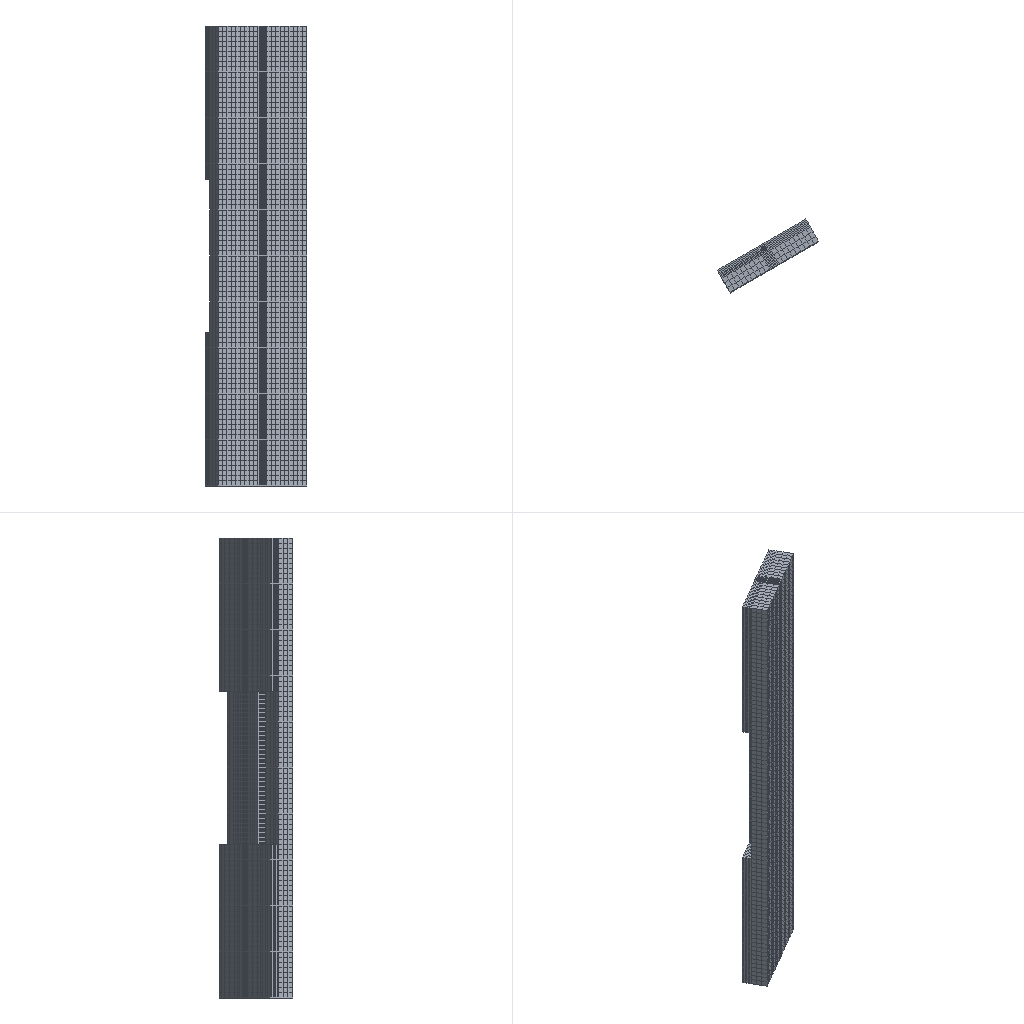Simulation study | abaqus
Set-up summary:
category,name,step,type,value,unit,region
solver,abaqus
solver,version,,,Abaqus/Standard 2020
units,not stated in the deck,,not stated
analysis,deck,,transient,transient
load_step,Gravity,Gravity,transient
load_step,requested,,,1
mesh,nodes,,,35489
mesh,elements,,,27780
element_type,C3D8,,solid,27780
load,load commands in deck,,count,3
bc,support commands in deck,,count,13
material,MAT-HUACHUANG,,in results
material,MAT-PIPE,,in results
material,MATE-HUATI,,in results
check,setup vs results,,match,"per instance, exact: element labels, types and connectivity; labels of the nodes the elements use; coordinates of those nodes at SINGLE_PRECISION in 3 of 3 instance(s)"
Abaqus input file, long lists of numbers shortened:
*Heading
** Job name: Job-1 Model name: Model-1
** Generated by: Abaqus/CAE 2020
*Preprint, echo=NO, model=NO, history=NO, contact=NO
**
** PARTS
**
*Part, name=huachuang
*End Part
**
*Part, name=huati
*End Part
**
*Part, name=pipe
*End Part
**
**
** ASSEMBLY
**
*Assembly, name=Assembly
**
*Instance, name=huachuang-1, part=huachuang
          0.,           0.,           0.
          0.,           0.,           0.,           0.,           0., 1., 30.
*Node
      1,           7.,   8.2,         120.
      2,           7.,   8.2,         180.
** (21823 more lines like these left out)
*Element, type=C3D8
  1,   246,  2747, 12140,  2715,     1,    95,  2251,   168
  2,  2747,  2748, 12141, 12140,    95,    96,  2252,  2251
** (17698 more lines like these left out)
*Nset, nset=_PickedSet97, internal, generate
     1,  21825,      1
*Elset, elset=_PickedSet97, internal, generate
     1,  17700,      1
*Elset, elset=_Surf-huachuang_S2, internal
  8191,  8192,  8193,  8194,  8195,  8196,  8197,  8198,  8199,  8200,  8201,  8202,  8203,  8204,  8205,  8206
  8207,  8208,  8209,  8210,  8211,  8212,  8213,  8214,  8215,  8216,  8217,  8218,  8219,  8220,  8221,  8222
** (21 more lines like these left out)
*Elset, elset=_Surf-huachuang_S5, internal
 3961, 3962, 3963, 3964, 3965, 3966, 3967, 3968, 3969, 3970, 3971, 3972, 3973, 3974, 3975, 3976
 3977, 3978, 3979, 3980, 3981, 3982, 3983, 3984, 3985, 3986, 3987, 3988, 3989, 3990, 4231, 4232
** (4 more lines like these left out)
*Surface, type=ELEMENT, name=Surf-huachuang
_Surf-huachuang_S2, S2
_Surf-huachuang_S5, S5
** Section: Section-huachuang
*Solid Section, elset=_PickedSet97, material=Mat-huachuang
,
*End Instance
**
*Instance, name=pipe-1, part=pipe
0.2301, 9.601,           0.
0.2301, 9.601,           0., 0.2301, 9.601, 1., 30.
*Node
      1,  0.5911,           0.,           0.
      2,  0.5911,           0.,         180.
** (2438 more lines like these left out)
*Element, type=C3D8
  1,    8,  203,  789,  267,    1,   19,  553,  144
  2,  203,  202,  790,  789,   19,   20,  554,  553
** (1198 more lines like these left out)
*Nset, nset=Set-pipe, generate
    1,  2440,     1
*Elset, elset=Set-pipe, generate
    1,  1200,     1
** Section: Section-pipe
*Solid Section, elset=Set-pipe, material=Mat-pipe
,
*End Instance
**
*Instance, name=huati-1, part=huati
          0.,           0.,           0.
          0.,           0.,           0.,           0.,           0., 1., 30.
*Node
      1,           7.,          10.,         120.
      2,           7.,   8.2,         120.
** (11222 more lines like these left out)
*Element, type=C3D8
  1, 1393, 1394, 6416, 6387,   66,   67, 1268, 1267
  2, 1394, 1395, 6415, 6416,   67,   68, 1269, 1268
** (8878 more lines like these left out)
*Nset, nset=Set-23, generate
     1,  11224,      1
*Elset, elset=Set-23, generate
    1,  8880,     1
** Section: Section-huati
*Solid Section, elset=Set-23, material=Mate-huati
,
*End Instance
**
*Nset, nset=Set-9, instance=pipe-1, generate
    1,  2440,     1
*Elset, elset=Set-9, instance=pipe-1, generate
    1,  1200,     1
*Nset, nset=Set-Huati, instance=huati-1, generate
     1,  11224,      1
*Elset, elset=Set-Huati, instance=huati-1, generate
    1,  8880,     1
*Nset, nset=Set-Huati-Side, instance=huati-1
    1,    2,    3,    4,    5,    6,    7,    8,    9,   10,   11,   12,   13,   14,   15,   16
   17,   18,   19,   20,   21,   22,   23,   24,   25,   26,   27,   28,   29,   30,   31,   32
** (21 more lines like these left out)
*Elset, elset=Set-Huati-Side, instance=huati-1
   30,   31,   32,  120,  150,  151,  181,  182,  183,  271,  272,  273,  274,  275,  276,  451
  452,  453,  454,  571,  572,  573,  661,  662,  663,  664,  781,  782,  783,  784,  785,  786
** (17 more lines like these left out)
*Nset, nset=Set-cemian, instance=huachuang-1
     2,     3,     5,     6,    10,    11,    13,    14,    22,    23,    25,    28,    29,    30,    31,    32
    34,    35,    38,    39,    42,    44,    46,    47,    48,    49,    50,    55,    58,    59,    62,    64
** (36 more lines like these left out)
*Nset, nset=Set-cemian, instance=pipe-1
   1,   2,   3,   4,   5,   6,   7,   8,   9,  10,  11,  12,  13,  14,  15,  16
  17,  18,  78,  79,  80,  81, 141, 142, 143, 144, 204, 205, 206, 207, 267, 268
** (3 more lines like these left out)
*Elset, elset=Set-cemian, instance=huachuang-1
    30,    60,    90,   120,   150,   180,   210,   240,   270,   300,   330,   360,   390,   420,   450,   480
   510,   540,   570,   600,   630,   660,   690,   720,   750,   780,   810,   840,   870,   900,   930,   960
** (30 more lines like these left out)
*Elset, elset=Set-cemian, instance=pipe-1
    1,   60,   61,  120,  121,  180,  181,  240,  241,  300,  301,  360,  361,  420,  421,  480
  481,  540,  541,  600,  601,  660,  661,  720,  721,  780,  781,  840,  841,  900,  901,  960
** (1 more lines like these left out)
*Nset, nset=Set-dimian, instance=huachuang-1
    17,    18,    19,    20,    29,    30,    31,    32,    47,    50,    51,    54,    59,    60,    61,    62
    87,    88,    91,    92,   465,   466,   467,   468,   469,   470,   471,   472,   473,   474,   475,   476
** (152 more lines like these left out)
*Elset, elset=Set-dimian, instance=huachuang-1
  2161,  2162,  2163,  2164,  2165,  2166,  2167,  2168,  2169,  2170,  2171,  2172,  2173,  2174,  2175,  2176
  2177,  2178,  2179,  2180,  2181,  2182,  2183,  2184,  2185,  2186,  2187,  2188,  2189,  2190,  2191,  2192
** (145 more lines like these left out)
*Nset, nset=Set-load, instance=huati-1
   11,   12,   15,   16,   35,   36,  358,  359,  360,  361,  362,  363,  364,  365,  366,  367
  368,  369,  370,  371,  372,  373,  374,  375,  376,  377,  378,  379,  380,  381,  382,  383
** (29 more lines like these left out)
*Elset, elset=Set-load, instance=huati-1
  961,  962,  963,  964,  965,  966,  967,  968,  969,  970,  971,  972,  973,  974,  975,  976
  977,  978,  979,  980,  981,  982,  983,  984,  985,  986,  987,  988,  989,  990,  991,  992
** (25 more lines like these left out)
*Nset, nset=Set-qianmian, instance=huachuang-1
     3,     4,     6,     7,    11,    12,    14,    15,    18,    19,    30,    32,    35,    36,    69,    70
    71,    72,    73,    74,    75,    76,    82,    83,    87,    88,    89,    90,    91,    92,    93,    94
** (92 more lines like these left out)
*Elset, elset=Set-qianmian, instance=huachuang-1
   241,   242,   243,   244,   245,   246,   247,   248,   249,   250,   251,   252,   253,   254,   255,   256
   257,   258,   259,   260,   261,   262,   263,   264,   265,   266,   267,   268,   269,   270,   511,   512
** (79 more lines like these left out)
*Nset, nset=huachuang, instance=huachuang-1, generate
     1,  21825,      1
*Elset, elset=huachuang, instance=huachuang-1, generate
     1,  17700,      1
*Nset, nset=model-all, instance=huachuang-1, generate
     1,  21825,      1
*Nset, nset=model-all, instance=pipe-1, generate
    1,  2440,     1
*Nset, nset=model-all, instance=huati-1, generate
     1,  11224,      1
*Elset, elset=model-all, instance=huachuang-1, generate
     1,  17700,      1
*Elset, elset=model-all, instance=pipe-1, generate
    1,  1200,     1
*Elset, elset=model-all, instance=huati-1, generate
    1,  8880,     1
*Elset, elset=_Huachuang-mid-top_S2, internal, instance=huachuang-1
  1621,  1622,  1623,  1624,  1625,  1626,  1627,  1628,  1629,  1630,  1631,  1632,  1633,  1634,  1635,  1636
  1637,  1638,  1639,  1640,  1641,  1642,  1643,  1644,  1645,  1646,  1647,  1648,  1649,  1650,  1651,  1652
** (23 more lines like these left out)
*Elset, elset=_Huachuang-mid-top_S6, internal, instance=huachuang-1, generate
 13171,  13978,      3
*Elset, elset=_Huachuang-mid-top_S1, internal, instance=huachuang-1, generate
 7261,  7380,     1
*Surface, type=ELEMENT, name=Huachuang-mid-top
_Huachuang-mid-top_S2, S2
_Huachuang-mid-top_S6, S6
_Huachuang-mid-top_S1, S1
*Elset, elset=_Huati-bottom_S2, internal, instance=huati-1
  961,  962,  963,  964,  965,  966,  967,  968,  969,  970,  971,  972,  973,  974,  975,  976
  977,  978,  979,  980,  981,  982,  983,  984,  985,  986,  987,  988,  989,  990,  991,  992
** (43 more lines like these left out)
*Elset, elset=_Huati-bottom_S3, internal, instance=huati-1
 5101, 5102, 5103, 5104, 5105, 5106, 5107, 5108, 5109, 5110, 5111, 5112, 5113, 5114, 5115, 5116
 5117, 5118, 5119, 5120, 5121, 5122, 5123, 5124, 5125, 5126, 5127, 5128, 5129, 5130, 5131, 5132
** (10 more lines like these left out)
*Elset, elset=_Huati-bottom_S4, internal, instance=huati-1
 4801, 4802, 4803, 4804, 4805, 4806, 4807, 4808, 4809, 4810, 4811, 4812, 4813, 4814, 4815, 4816
 4817, 4818, 4819, 4820, 4821, 4822, 4823, 4824, 4825, 4826, 4827, 4828, 4829, 4830, 4831, 4832
** (10 more lines like these left out)
*Surface, type=ELEMENT, name=Huati-bottom
_Huati-bottom_S2, S2
_Huati-bottom_S3, S3
_Huati-bottom_S4, S4
*Elset, elset=_Surf-13_S2, internal, instance=pipe-1, generate
 301,  900,    1
*Surface, type=ELEMENT, name=Surf-13
_Surf-13_S2, S2
*Elset, elset=_Surf-LOAD_S3, internal, instance=huati-1
  961,  962,  963,  964,  965,  966,  967,  968,  969,  970,  971,  972,  973,  974,  975,  976
  977,  978,  979,  980,  981,  982,  983,  984,  985,  986,  987,  988,  989,  990,  991,  992
** (25 more lines like these left out)
*Surface, type=ELEMENT, name=Surf-LOAD
_Surf-LOAD_S3, S3
*Elset, elset=_Surf-huachuang_S4, internal, instance=huachuang-1
  9392,  9394,  9396,  9398,  9400,  9402,  9404,  9406,  9408,  9410,  9412,  9414,  9416,  9418,  9420,  9422
  9424,  9426,  9428,  9430,  9432,  9434,  9436,  9438,  9440,  9442,  9444,  9446,  9448,  9450, 10562, 10564
** (18 more lines like these left out)
*Elset, elset=_Surf-huachuang_S3, internal, instance=huachuang-1
  9331,  9332,  9333,  9334,  9335,  9336,  9337,  9338,  9339,  9340,  9341,  9342,  9343,  9344,  9345,  9361
  9362,  9363,  9364,  9365,  9366,  9367,  9368,  9369,  9370,  9371,  9372,  9373,  9374,  9375,  9481,  9482
** (16 more lines like these left out)
*Elset, elset=_Surf-huachuang_S2, internal, instance=huachuang-1
  2431,  2432,  2433,  2434,  2435,  2436,  2437,  2438,  2439,  2440,  2441,  2442,  2443,  2444,  2445,  2446
  2447,  2448,  2449,  2450,  2451,  2452,  2453,  2454,  2455,  2456,  2457,  2458,  2459,  2460,  2461,  2462
** (35 more lines like these left out)
*Elset, elset=_Surf-huachuang_S6, internal, instance=huachuang-1, generate
 12931,  13019,      2
*Surface, type=ELEMENT, name=Surf-huachuang
_Surf-huachuang_S4, S4
_Surf-huachuang_S3, S3
_Surf-huachuang_S2, S2
_Surf-huachuang_S6, S6
*Elset, elset=_Surf-huati_S3, internal, instance=huati-1
  451,  452,  455,  456,  459,  460,  463,  464,  467,  468,  471,  472,  475,  476,  479,  480
  483,  484,  487,  488,  491,  492,  495,  496,  499,  500,  503,  504,  507,  508,  511,  512
** (42 more lines like these left out)
*Elset, elset=_Surf-huati_S4, internal, instance=huati-1
  272,  274,  276,  278,  280,  282,  284,  286,  288,  290,  292,  294,  296,  298,  300,  302
  304,  306,  308,  310,  312,  314,  316,  318,  320,  322,  324,  326,  328,  330,  332,  334
** (30 more lines like these left out)
*Surface, type=ELEMENT, name=Surf-huati
_Surf-huati_S3, S3
_Surf-huati_S4, S4
*Elset, elset=_Surf-pipe_S1, internal, instance=pipe-1, generate
    1,  1200,     1
*Surface, type=ELEMENT, name=Surf-pipe
_Surf-pipe_S1, S1
*Elset, elset=_huachuang-left-side_S3, internal, instance=huachuang-1
  5341,  5342,  5343,  5386,  5387,  5388,  5641,  5656,  5671,  5731,  5761,  5762,  9301,  9316,  9451, 10471
 10486, 10501, 10741, 14821, 14822, 15121, 15122, 15151, 15152, 16891, 16892, 16893, 16981, 16982, 16983, 17071
** (2 more lines like these left out)
*Elset, elset=_huachuang-left-side_S4, internal, instance=huachuang-1
  5595,  5610,  5625,  5640,  8220,  8250,  8280,  8310,  8340,  8370,  8400,  8430,  8460,  8490,  8520,  8550
  8580,  8610,  8640,  8670,  8700,  8730,  8760,  8790,  8820,  8850,  8880,  8910,  8940,  8970,  9000,  9030
** (2 more lines like these left out)
*Elset, elset=_huachuang-left-side_S2, internal, instance=huachuang-1
  9481,  9482,  9483,  9484,  9485,  9486,  9571,  9572,  9573, 10771, 10772, 10773, 10774, 10775, 10776, 10861
 10862, 10863, 15181, 15182, 15183, 15184, 15185, 15186
*Elset, elset=_huachuang-left-side_S6, internal, instance=huachuang-1
    1,   31,   61,   91,  121,  151,  181,  211,  241,  271,  301,  331,  361,  391,  421,  451
  481,  511,  541,  571,  601,  631,  661,  691,  721,  751,  781, 4531, 4561, 4591, 4621, 4651
** (2 more lines like these left out)
*Surface, type=ELEMENT, name=huachuang-left-side
_huachuang-left-side_S3, S3
_huachuang-left-side_S4, S4
_huachuang-left-side_S2, S2
_huachuang-left-side_S6, S6
*Elset, elset=_huachuang-right-side_S3, internal, instance=huachuang-1
  2431,  2432,  2433,  2476,  2477,  2478,  2776,  2791,  2806,  6721,  6722,  6751,  6752, 12211, 12226, 12391
 12721, 12722, 13021, 13022, 13051, 13052
*Elset, elset=_huachuang-right-side_S4, internal, instance=huachuang-1
  2685,  2700,  2715,  2730,  6645,  6660,  6675,  6690,  6705,  6720,  6900,  6915,  6930,  7410,  7440,  7470
  7500,  7530,  7560,  7590,  7620,  7650,  7680,  7710,  7740,  7770,  7800,  7830,  7860,  7890,  7920,  7950
** (3 more lines like these left out)
*Elset, elset=_huachuang-right-side_S2, internal, instance=huachuang-1
  2821,  2822,  2851,  6931,  6946,  6947, 12421, 12422, 12423, 12424, 12425, 12426, 12511, 12512, 12513, 13081
 13082, 13083, 13084, 13085, 13086
*Elset, elset=_huachuang-right-side_S6, internal, instance=huachuang-1
   811,   841,   871,   901,   931,   961,   991,  1021,  1051,  1081,  1111,  1141,  1171,  1201,  1231,  1261
  1291,  1321,  1351,  1381,  1411,  1441,  1471,  1501,  1531,  1561,  1591, 13981, 14011, 14041, 14071, 14101
** (2 more lines like these left out)
*Surface, type=ELEMENT, name=huachuang-right-side
_huachuang-right-side_S3, S3
_huachuang-right-side_S4, S4
_huachuang-right-side_S2, S2
_huachuang-right-side_S6, S6
*Elset, elset=_huati-left-side_S4, internal, instance=huati-1
   30, 1020, 1080, 1140, 1200, 1260, 1320, 1380, 1440, 1500, 1560, 1620, 1680, 1740, 1800, 1860
 1920, 1980, 2040, 2100, 2160, 2220, 2280, 2340, 2400, 3960, 3990, 5130, 5160, 5490, 5520, 5550
** (2 more lines like these left out)
*Elset, elset=_huati-left-side_S3, internal, instance=huati-1
   31,   32, 3991, 4411, 4412, 4413, 4981, 4982, 5041, 5042, 5551, 8221, 8251, 8611, 8612, 8613
*Elset, elset=_huati-left-side_S2, internal, instance=huati-1
  181,  182,  183,  271,  272,  273,  274,  275,  276,  451,  452,  453,  454, 4501, 4502, 4503
 4504, 4621, 4622, 4623, 4624, 4625, 4626, 8701, 8702, 8703, 8704, 8705, 8706
*Elset, elset=_huati-left-side_S6, internal, instance=huati-1
 2401, 2461, 2521, 2581, 2641, 2701, 2761, 2821, 2881, 2941, 3001, 3061, 3121, 3181, 3241, 3301
 3361, 3421, 3481, 3541, 3601, 3661, 3721, 3781, 6841, 6901, 6961, 7021, 7081, 7141, 7201, 7261
** (1 more lines like these left out)
*Surface, type=ELEMENT, name=huati-left-side
_huati-left-side_S4, S4
_huati-left-side_S3, S3
_huati-left-side_S2, S2
_huati-left-side_S6, S6
*Elset, elset=_huati-right-side_S4, internal, instance=huati-1
  120,  150, 2460, 2520, 2580, 2640, 2700, 2760, 2820, 2880, 2940, 3000, 3060, 3120, 3180, 3240
 3300, 3360, 3420, 3480, 3540, 3600, 3660, 3720, 3780, 3840, 3870, 4890, 4920, 4950, 4980, 6900
** (2 more lines like these left out)
*Elset, elset=_huati-right-side_S6, internal, instance=huati-1
  961, 1021, 1081, 1141, 1201, 1261, 1321, 1381, 1441, 1501, 1561, 1621, 1681, 1741, 1801, 1861
 1921, 1981, 2041, 2101, 2161, 2221, 2281, 2341, 5761, 5821, 5881, 5941, 6001, 6061, 6121, 6181
** (1 more lines like these left out)
*Elset, elset=_huati-right-side_S3, internal, instance=huati-1
  151,  571,  572,  573, 3871, 3872, 4801, 4831, 7981, 7982, 8041, 8042
*Elset, elset=_huati-right-side_S2, internal, instance=huati-1
  661,  662,  663,  664,  781,  782,  783,  784,  785,  786, 4021, 4022, 4023, 4111, 4112, 4113
 4114, 4115, 4116, 4291, 4292, 4293, 4294, 5161, 5162, 5163, 5164, 5165, 5166, 5341, 5342, 5343
** (1 more lines like these left out)
*Surface, type=ELEMENT, name=huati-right-side
_huati-right-side_S4, S4
_huati-right-side_S6, S6
_huati-right-side_S2, S2
_huati-right-side_S3, S3
*Elset, elset=_pipe-inner_S2, internal, instance=pipe-1, generate
    1,  1200,     1
*Surface, type=ELEMENT, name=pipe-inner
_pipe-inner_S2, S2
*End Assembly
*Amplitude, name=Amp-1
             0.,              0.,              1.,              1.
**
** MATERIALS
**
*Material, name=Mat-huachuang
*Density
1800.,
*Elastic
 3.2e+06, 0.28
*Mohr Coulomb
20., 0.1
*Mohr Coulomb Hardening
 2e+07,0.
*Material, name=Mat-pipe
*Density
7900.,
*Elastic
 2.1e+11, 0.3
*Expansion
 1.25e-05,
*Plastic
 4.60095e+08,          0.
 4.67441e+08,    8.87e-06
 4.74118e+08,    1.63e-05
 4.80796e+08,    2.73e-05
 4.87474e+08,    4.35e-05
 4.94152e+08,    6.72e-05
 5.00829e+08, 0.0001015
 5.07507e+08, 0.000151
 5.14185e+08,   0.0002218
 5.20862e+08, 0.0003226
  5.2754e+08, 0.000465
 5.34218e+08, 0.0006646
 5.40896e+08, 0.0009423
 5.47573e+08,  0.001325
 5.54251e+08,   0.001846
 5.60929e+08,  0.002547
 5.67607e+08,  0.003475
 5.74284e+08,  0.004684
 5.80962e+08,  0.006226
  5.8764e+08,  0.008154
 5.94317e+08,   0.01051
 6.00995e+08,   0.01331
 6.07673e+08,   0.01658
 6.14351e+08,   0.02031
 6.21028e+08,   0.02448
 6.27706e+08,   0.02906
 6.34384e+08,   0.03401
 6.41061e+08,   0.03929
 6.47739e+08,   0.04486
 6.54417e+08,   0.05071
 6.61095e+08,   0.05683
 6.67772e+08,   0.06302
*Material, name=Mate-huati
*Density
1800.,
*Elastic
 3.115e+06, 0.3
*Mohr Coulomb
20., 0.1
*Mohr Coulomb Hardening
 2e+07,0.
**
** INTERACTION PROPERTIES
**
*Surface Interaction, name=IntProp-1
1.,
*Friction, slip tolerance=0.005
 0.3,
*Surface Behavior, pressure-overclosure=HARD
**
** BOUNDARY CONDITIONS
**
** Name: huachuang-cemian Type: Displacement/rotation angle
*Boundary
Set-cemian, 1, 1
Set-cemian, 3, 3
** Name: huachuang-dimian Type: Displacement/rotation angle
*Boundary
Set-dimian, 1, 1
Set-dimian, 2, 2
Set-dimian, 3, 3
** Name: huachuang-qianmian Type: Displacement/rotation angle
*Boundary
Set-qianmian, 1, 1
** Name: huati-beimian Type: Displacement/rotation angle
*Boundary
Set-load, 1, 1
**
** PREDEFINED FIELDS
**
** Name: Predefined Field-1   Type: Temperature
*Initial Conditions, type=TEMPERATURE
Set-9, 0.
**
** INTERACTIONS
**
** Interaction: Huachuang-Huati
*Contact Pair, interaction=IntProp-1, type=SURFACE TO SURFACE
Huati-bottom, Huachuang-mid-top
** Interaction: huachuang-huati-left-side
*Contact Pair, interaction=IntProp-1, type=SURFACE TO SURFACE
huati-left-side, huachuang-left-side
** Interaction: huachuang-huati-right-side
*Contact Pair, interaction=IntProp-1, type=SURFACE TO SURFACE
huati-right-side, huachuang-right-side
** Interaction: pipe-huachuang
*Contact Pair, interaction=IntProp-1, type=SURFACE TO SURFACE
Surf-huachuang, Surf-pipe
** Interaction: pipe-huati
*Contact Pair, interaction=IntProp-1, type=SURFACE TO SURFACE
Surf-huati, Surf-pipe
** ----------------------------------------------------------------
**
** STEP: Gravity
**
*Step, name=Gravity, nlgeom=YES, inc=10000, unsymm=YES
*Dynamic
0.001,1.,1e-05
**
** BOUNDARY CONDITIONS
**
** Name: huachuang-cemian Type: Displacement/rotation angle
*Boundary, op=NEW
Set-cemian, 1, 1
Set-cemian, 3, 3
** Name: huachuang-dimian Type: Displacement/rotation angle
*Boundary, op=NEW
Set-dimian, 1, 1
Set-dimian, 2, 2
Set-dimian, 3, 3
** Name: huachuang-qianmian Type: Displacement/rotation angle
*Boundary, op=NEW
Set-qianmian, 1, 1
** Name: huati-beimian Type: Displacement/rotation angle
*Boundary, op=NEW
**
** LOADS
**
** Name: Gravity   Type: Gravity
*Dload
model-all, GRAV, 9.8, 0., -1., 0.
** Name: Load-p   Type: Pressure
*Dsload, amplitude=Amp-1
Surf-13, P, 100000.
**
** PREDEFINED FIELDS
**
** Name: Predefined Field-1   Type: Temperature
*Temperature
Set-9, 30.
**
** OUTPUT REQUESTS
**
*Restart, write, frequency=0
**
** FIELD OUTPUT: F-Output-1
**
*Output, field, frequency=1
*Node Output
CF, RF, RM, RT, U, V
*Element Output, directions=YES
E, LE, MISES, NFORC, PE, PEEQ, PEMAG, S
*Contact Output
CDISP, CSTRESS
*Output, history, frequency=0
*End Step
Results summary:
result,step,,completed,increments=21 time=1.0/1.0
result,analysis,,,transient
result,last_loadstep,,,1
result,primary field,,,U
result,reaction total,,FX,54897522.404,model units
result,reaction total,,FY,844177796.895,model units
result,reaction total,,FZ,-12292.208,model units